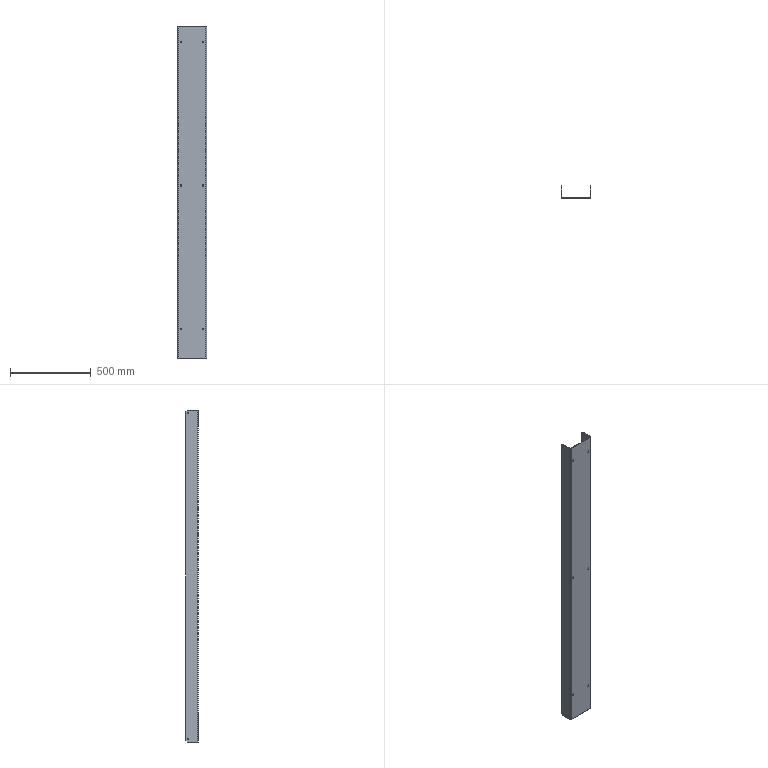Part | STEP file | HXGR200008-05-10 | 1 solid | 46 faces | box 180 x 80 x 2050 mm | volume 1362117 mm3 | cylinder 24 | plane 22 | commonest cylinder face diameters 8 x20 6 x2 10 x2
STEP:
#1=CARTESIAN_POINT('',(88.,25.,-1009.));
#2=VERTEX_POINT('',#1);
#3=CARTESIAN_POINT('',(88.,25.,-1001.));
#4=VERTEX_POINT('',#3);
#5=CARTESIAN_POINT('',(88.,25.,-1005.));
#6=DIRECTION('',(-1.,0.,0.));
#7=DIRECTION('',(0.,0.,1.));
#8=AXIS2_PLACEMENT_3D('',#5,#6,#7);
#9=CIRCLE('',#8,4.);
#10=EDGE_CURVE('',#2,#4,#9,.T.);
#11=ORIENTED_EDGE('',*,*,#10,.T.);
#12=CARTESIAN_POINT('',(90.,25.,-1001.));
#13=VERTEX_POINT('',#12);
#14=CARTESIAN_POINT('',(90.,25.,-1001.));
#15=DIRECTION('',(1.,0.,0.));
#16=VECTOR('',#15,1000.);
#17=LINE('',#14,#16);
#18=EDGE_CURVE('',#4,#13,#17,.T.);
#19=ORIENTED_EDGE('',*,*,#18,.T.);
#20=CARTESIAN_POINT('',(90.,25.,-1009.));
#21=VERTEX_POINT('',#20);
#22=CARTESIAN_POINT('',(90.,25.,-1005.));
#23=DIRECTION('',(1.,0.,0.));
#24=DIRECTION('',(0.,0.,-1.));
#25=AXIS2_PLACEMENT_3D('',#22,#23,#24);
#26=CIRCLE('',#25,4.);
#27=EDGE_CURVE('',#13,#21,#26,.T.);
#28=ORIENTED_EDGE('',*,*,#27,.T.);
#29=CARTESIAN_POINT('',(90.,25.,-1009.));
#30=DIRECTION('',(1.,0.,0.));
#31=VECTOR('',#30,1000.);
#32=LINE('',#29,#31);
#33=EDGE_CURVE('',#2,#21,#32,.T.);
#34=ORIENTED_EDGE('',*,*,#33,.F.);
#35=EDGE_LOOP('',(#11,#19,#28,#34));
#36=FACE_OUTER_BOUND('',#35,.T.);
#37=CARTESIAN_POINT('',(90.,25.,-1005.));
#38=DIRECTION('',(1.,0.,0.));
#39=DIRECTION('',(0.,0.,-1.));
#40=AXIS2_PLACEMENT_3D('',#37,#38,#39);
#41=CYLINDRICAL_SURFACE('',#40,4.);
#42=ADVANCED_FACE('',(#36),#41,.F.);
#43=CARTESIAN_POINT('',(-90.,25.,-1001.));
#44=VERTEX_POINT('',#43);
#45=CARTESIAN_POINT('',(-90.,25.,-1009.));
#46=VERTEX_POINT('',#45);
#47=CARTESIAN_POINT('',(-90.,25.,-1005.));
#48=DIRECTION('',(1.,0.,0.));
#49=DIRECTION('',(0.,0.,-1.));
#50=AXIS2_PLACEMENT_3D('',#47,#48,#49);
#51=CIRCLE('',#50,4.);
#52=EDGE_CURVE('',#44,#46,#51,.T.);
#53=ORIENTED_EDGE('',*,*,#52,.F.);
#54=CARTESIAN_POINT('',(-88.,25.,-1001.));
#55=VERTEX_POINT('',#54);
#56=CARTESIAN_POINT('',(90.,25.,-1001.));
#57=DIRECTION('',(1.,0.,0.));
#58=VECTOR('',#57,1000.);
#59=LINE('',#56,#58);
#60=EDGE_CURVE('',#44,#55,#59,.T.);
#61=ORIENTED_EDGE('',*,*,#60,.T.);
#62=CARTESIAN_POINT('',(-88.,25.,-1009.));
#63=VERTEX_POINT('',#62);
#64=CARTESIAN_POINT('',(-88.,25.,-1005.));
#65=DIRECTION('',(1.,0.,0.));
#66=DIRECTION('',(0.,0.,-1.));
#67=AXIS2_PLACEMENT_3D('',#64,#65,#66);
#68=CIRCLE('',#67,4.);
#69=EDGE_CURVE('',#55,#63,#68,.T.);
#70=ORIENTED_EDGE('',*,*,#69,.T.);
#71=CARTESIAN_POINT('',(90.,25.,-1009.));
#72=DIRECTION('',(1.,0.,0.));
#73=VECTOR('',#72,1000.);
#74=LINE('',#71,#73);
#75=EDGE_CURVE('',#46,#63,#74,.T.);
#76=ORIENTED_EDGE('',*,*,#75,.F.);
#77=EDGE_LOOP('',(#53,#61,#70,#76));
#78=FACE_OUTER_BOUND('',#77,.T.);
#79=CARTESIAN_POINT('',(90.,25.,-1005.));
#80=DIRECTION('',(1.,0.,0.));
#81=DIRECTION('',(0.,0.,-1.));
#82=AXIS2_PLACEMENT_3D('',#79,#80,#81);
#83=CYLINDRICAL_SURFACE('',#82,4.);
#84=ADVANCED_FACE('',(#78),#83,.F.);
#85=CARTESIAN_POINT('',(88.,25.,1001.));
#86=VERTEX_POINT('',#85);
#87=CARTESIAN_POINT('',(88.,25.,1009.));
#88=VERTEX_POINT('',#87);
#89=CARTESIAN_POINT('',(88.,25.,1005.));
#90=DIRECTION('',(-1.,0.,0.));
#91=DIRECTION('',(0.,0.,1.));
#92=AXIS2_PLACEMENT_3D('',#89,#90,#91);
#93=CIRCLE('',#92,4.);
#94=EDGE_CURVE('',#86,#88,#93,.T.);
#95=ORIENTED_EDGE('',*,*,#94,.T.);
#96=CARTESIAN_POINT('',(90.,25.,1009.));
#97=VERTEX_POINT('',#96);
#98=CARTESIAN_POINT('',(90.,25.,1009.));
#99=DIRECTION('',(1.,0.,0.));
#100=VECTOR('',#99,1000.);
#101=LINE('',#98,#100);
#102=EDGE_CURVE('',#88,#97,#101,.T.);
#103=ORIENTED_EDGE('',*,*,#102,.T.);
#104=CARTESIAN_POINT('',(90.,25.,1001.));
#105=VERTEX_POINT('',#104);
#106=CARTESIAN_POINT('',(90.,25.,1005.));
#107=DIRECTION('',(1.,0.,0.));
#108=DIRECTION('',(0.,0.,-1.));
#109=AXIS2_PLACEMENT_3D('',#106,#107,#108);
#110=CIRCLE('',#109,4.);
#111=EDGE_CURVE('',#97,#105,#110,.T.);
#112=ORIENTED_EDGE('',*,*,#111,.T.);
#113=CARTESIAN_POINT('',(90.,25.,1001.));
#114=DIRECTION('',(1.,0.,0.));
#115=VECTOR('',#114,1000.);
#116=LINE('',#113,#115);
#117=EDGE_CURVE('',#86,#105,#116,.T.);
#118=ORIENTED_EDGE('',*,*,#117,.F.);
#119=EDGE_LOOP('',(#95,#103,#112,#118));
#120=FACE_OUTER_BOUND('',#119,.T.);
#121=CARTESIAN_POINT('',(90.,25.,1005.));
#122=DIRECTION('',(1.,0.,0.));
#123=DIRECTION('',(0.,0.,-1.));
#124=AXIS2_PLACEMENT_3D('',#121,#122,#123);
#125=CYLINDRICAL_SURFACE('',#124,4.);
#126=ADVANCED_FACE('',(#120),#125,.F.);
#127=CARTESIAN_POINT('',(-90.,25.,1009.));
#128=VERTEX_POINT('',#127);
#129=CARTESIAN_POINT('',(-90.,25.,1001.));
#130=VERTEX_POINT('',#129);
#131=CARTESIAN_POINT('',(-90.,25.,1005.));
#132=DIRECTION('',(1.,0.,0.));
#133=DIRECTION('',(0.,0.,-1.));
#134=AXIS2_PLACEMENT_3D('',#131,#132,#133);
#135=CIRCLE('',#134,4.);
#136=EDGE_CURVE('',#128,#130,#135,.T.);
#137=ORIENTED_EDGE('',*,*,#136,.F.);
#138=CARTESIAN_POINT('',(-88.,25.,1009.));
#139=VERTEX_POINT('',#138);
#140=CARTESIAN_POINT('',(90.,25.,1009.));
#141=DIRECTION('',(1.,0.,0.));
#142=VECTOR('',#141,1000.);
#143=LINE('',#140,#142);
#144=EDGE_CURVE('',#128,#139,#143,.T.);
#145=ORIENTED_EDGE('',*,*,#144,.T.);
#146=CARTESIAN_POINT('',(-88.,25.,1001.));
#147=VERTEX_POINT('',#146);
#148=CARTESIAN_POINT('',(-88.,25.,1005.));
#149=DIRECTION('',(1.,0.,0.));
#150=DIRECTION('',(0.,0.,-1.));
#151=AXIS2_PLACEMENT_3D('',#148,#149,#150);
#152=CIRCLE('',#151,4.);
#153=EDGE_CURVE('',#139,#147,#152,.T.);
#154=ORIENTED_EDGE('',*,*,#153,.T.);
#155=CARTESIAN_POINT('',(90.,25.,1001.));
#156=DIRECTION('',(1.,0.,0.));
#157=VECTOR('',#156,1000.);
#158=LINE('',#155,#157);
#159=EDGE_CURVE('',#130,#147,#158,.T.);
#160=ORIENTED_EDGE('',*,*,#159,.F.);
#161=EDGE_LOOP('',(#137,#145,#154,#160));
#162=FACE_OUTER_BOUND('',#161,.T.);
#163=CARTESIAN_POINT('',(90.,25.,1005.));
#164=DIRECTION('',(1.,0.,0.));
#165=DIRECTION('',(0.,0.,-1.));
#166=AXIS2_PLACEMENT_3D('',#163,#164,#165);
#167=CYLINDRICAL_SURFACE('',#166,4.);
#168=ADVANCED_FACE('',(#162),#167,.F.);
#169=CARTESIAN_POINT('',(-67.5,-40.,-849.));
#170=VERTEX_POINT('',#169);
#171=CARTESIAN_POINT('',(-67.5,-40.,-841.));
#172=VERTEX_POINT('',#171);
#173=CARTESIAN_POINT('',(-67.5,-40.,-845.));
#174=DIRECTION('',(0.,1.,0.));
#175=DIRECTION('',(0.,0.,1.));
#176=AXIS2_PLACEMENT_3D('',#173,#174,#175);
#177=CIRCLE('',#176,4.);
#178=EDGE_CURVE('',#170,#172,#177,.T.);
#179=ORIENTED_EDGE('',*,*,#178,.F.);
#180=CARTESIAN_POINT('',(-67.5,-38.,-849.));
#181=VERTEX_POINT('',#180);
#182=CARTESIAN_POINT('',(-67.5,-38.,-849.));
#183=DIRECTION('',(0.,1.,0.));
#184=VECTOR('',#183,1000.);
#185=LINE('',#182,#184);
#186=EDGE_CURVE('',#170,#181,#185,.T.);
#187=ORIENTED_EDGE('',*,*,#186,.T.);
#188=CARTESIAN_POINT('',(-67.5,-38.,-841.));
#189=VERTEX_POINT('',#188);
#190=CARTESIAN_POINT('',(-67.5,-38.,-845.));
#191=DIRECTION('',(0.,1.,0.));
#192=DIRECTION('',(0.,0.,1.));
#193=AXIS2_PLACEMENT_3D('',#190,#191,#192);
#194=CIRCLE('',#193,4.);
#195=EDGE_CURVE('',#181,#189,#194,.T.);
#196=ORIENTED_EDGE('',*,*,#195,.T.);
#197=CARTESIAN_POINT('',(-67.5,-38.,-841.));
#198=DIRECTION('',(0.,1.,0.));
#199=VECTOR('',#198,1000.);
#200=LINE('',#197,#199);
#201=EDGE_CURVE('',#172,#189,#200,.T.);
#202=ORIENTED_EDGE('',*,*,#201,.F.);
#203=EDGE_LOOP('',(#179,#187,#196,#202));
#204=FACE_OUTER_BOUND('',#203,.T.);
#205=CARTESIAN_POINT('',(-67.5,-38.,-845.));
#206=DIRECTION('',(0.,1.,0.));
#207=DIRECTION('',(0.,0.,1.));
#208=AXIS2_PLACEMENT_3D('',#205,#206,#207);
#209=CYLINDRICAL_SURFACE('',#208,4.);
#210=ADVANCED_FACE('',(#204),#209,.F.);
#211=CARTESIAN_POINT('',(67.5,-40.,-849.));
#212=VERTEX_POINT('',#211);
#213=CARTESIAN_POINT('',(67.5,-40.,-841.));
#214=VERTEX_POINT('',#213);
#215=CARTESIAN_POINT('',(67.5,-40.,-845.));
#216=DIRECTION('',(0.,1.,0.));
#217=DIRECTION('',(0.,0.,1.));
#218=AXIS2_PLACEMENT_3D('',#215,#216,#217);
#219=CIRCLE('',#218,4.);
#220=EDGE_CURVE('',#212,#214,#219,.T.);
#221=ORIENTED_EDGE('',*,*,#220,.F.);
#222=CARTESIAN_POINT('',(67.5,-38.,-849.));
#223=VERTEX_POINT('',#222);
#224=CARTESIAN_POINT('',(67.5,-38.,-849.));
#225=DIRECTION('',(0.,1.,0.));
#226=VECTOR('',#225,1000.);
#227=LINE('',#224,#226);
#228=EDGE_CURVE('',#212,#223,#227,.T.);
#229=ORIENTED_EDGE('',*,*,#228,.T.);
#230=CARTESIAN_POINT('',(67.5,-38.,-841.));
#231=VERTEX_POINT('',#230);
#232=CARTESIAN_POINT('',(67.5,-38.,-845.));
#233=DIRECTION('',(0.,1.,0.));
#234=DIRECTION('',(0.,0.,1.));
#235=AXIS2_PLACEMENT_3D('',#232,#233,#234);
#236=CIRCLE('',#235,4.);
#237=EDGE_CURVE('',#223,#231,#236,.T.);
#238=ORIENTED_EDGE('',*,*,#237,.T.);
#239=CARTESIAN_POINT('',(67.5,-38.,-841.));
#240=DIRECTION('',(0.,1.,0.));
#241=VECTOR('',#240,1000.);
#242=LINE('',#239,#241);
#243=EDGE_CURVE('',#214,#231,#242,.T.);
#244=ORIENTED_EDGE('',*,*,#243,.F.);
#245=EDGE_LOOP('',(#221,#229,#238,#244));
#246=FACE_OUTER_BOUND('',#245,.T.);
#247=CARTESIAN_POINT('',(67.5,-38.,-845.));
#248=DIRECTION('',(0.,1.,0.));
#249=DIRECTION('',(0.,0.,1.));
#250=AXIS2_PLACEMENT_3D('',#247,#248,#249);
#251=CYLINDRICAL_SURFACE('',#250,4.);
#252=ADVANCED_FACE('',(#246),#251,.F.);
#253=CARTESIAN_POINT('',(-67.5,-40.,36.));
#254=VERTEX_POINT('',#253);
#255=CARTESIAN_POINT('',(-67.5,-40.,44.));
#256=VERTEX_POINT('',#255);
#257=CARTESIAN_POINT('',(-67.5,-40.,40.));
#258=DIRECTION('',(0.,1.,0.));
#259=DIRECTION('',(0.,0.,1.));
#260=AXIS2_PLACEMENT_3D('',#257,#258,#259);
#261=CIRCLE('',#260,4.);
#262=EDGE_CURVE('',#254,#256,#261,.T.);
#263=ORIENTED_EDGE('',*,*,#262,.F.);
#264=CARTESIAN_POINT('',(-67.5,-38.,36.));
#265=VERTEX_POINT('',#264);
#266=CARTESIAN_POINT('',(-67.5,-38.,36.));
#267=DIRECTION('',(0.,1.,0.));
#268=VECTOR('',#267,1000.);
#269=LINE('',#266,#268);
#270=EDGE_CURVE('',#254,#265,#269,.T.);
#271=ORIENTED_EDGE('',*,*,#270,.T.);
#272=CARTESIAN_POINT('',(-67.5,-38.,44.));
#273=VERTEX_POINT('',#272);
#274=CARTESIAN_POINT('',(-67.5,-38.,40.));
#275=DIRECTION('',(0.,1.,0.));
#276=DIRECTION('',(0.,0.,1.));
#277=AXIS2_PLACEMENT_3D('',#274,#275,#276);
#278=CIRCLE('',#277,4.);
#279=EDGE_CURVE('',#265,#273,#278,.T.);
#280=ORIENTED_EDGE('',*,*,#279,.T.);
#281=CARTESIAN_POINT('',(-67.5,-38.,44.));
#282=DIRECTION('',(0.,1.,0.));
#283=VECTOR('',#282,1000.);
#284=LINE('',#281,#283);
#285=EDGE_CURVE('',#256,#273,#284,.T.);
#286=ORIENTED_EDGE('',*,*,#285,.F.);
#287=EDGE_LOOP('',(#263,#271,#280,#286));
#288=FACE_OUTER_BOUND('',#287,.T.);
#289=CARTESIAN_POINT('',(-67.5,-38.,40.));
#290=DIRECTION('',(0.,1.,0.));
#291=DIRECTION('',(0.,0.,1.));
#292=AXIS2_PLACEMENT_3D('',#289,#290,#291);
#293=CYLINDRICAL_SURFACE('',#292,4.);
#294=ADVANCED_FACE('',(#288),#293,.F.);
#295=CARTESIAN_POINT('',(67.5,-40.,36.));
#296=VERTEX_POINT('',#295);
#297=CARTESIAN_POINT('',(67.5,-40.,44.));
#298=VERTEX_POINT('',#297);
#299=CARTESIAN_POINT('',(67.5,-40.,40.));
#300=DIRECTION('',(0.,1.,0.));
#301=DIRECTION('',(0.,0.,1.));
#302=AXIS2_PLACEMENT_3D('',#299,#300,#301);
#303=CIRCLE('',#302,4.);
#304=EDGE_CURVE('',#296,#298,#303,.T.);
#305=ORIENTED_EDGE('',*,*,#304,.F.);
#306=CARTESIAN_POINT('',(67.5,-38.,36.));
#307=VERTEX_POINT('',#306);
#308=CARTESIAN_POINT('',(67.5,-38.,36.));
#309=DIRECTION('',(0.,1.,0.));
#310=VECTOR('',#309,1000.);
#311=LINE('',#308,#310);
#312=EDGE_CURVE('',#296,#307,#311,.T.);
#313=ORIENTED_EDGE('',*,*,#312,.T.);
#314=CARTESIAN_POINT('',(67.5,-38.,44.));
#315=VERTEX_POINT('',#314);
#316=CARTESIAN_POINT('',(67.5,-38.,40.));
#317=DIRECTION('',(0.,1.,0.));
#318=DIRECTION('',(0.,0.,1.));
#319=AXIS2_PLACEMENT_3D('',#316,#317,#318);
#320=CIRCLE('',#319,4.);
#321=EDGE_CURVE('',#307,#315,#320,.T.);
#322=ORIENTED_EDGE('',*,*,#321,.T.);
#323=CARTESIAN_POINT('',(67.5,-38.,44.));
#324=DIRECTION('',(0.,1.,0.));
#325=VECTOR('',#324,1000.);
#326=LINE('',#323,#325);
#327=EDGE_CURVE('',#298,#315,#326,.T.);
#328=ORIENTED_EDGE('',*,*,#327,.F.);
#329=EDGE_LOOP('',(#305,#313,#322,#328));
#330=FACE_OUTER_BOUND('',#329,.T.);
#331=CARTESIAN_POINT('',(67.5,-38.,40.));
#332=DIRECTION('',(0.,1.,0.));
#333=DIRECTION('',(0.,0.,1.));
#334=AXIS2_PLACEMENT_3D('',#331,#332,#333);
#335=CYLINDRICAL_SURFACE('',#334,4.);
#336=ADVANCED_FACE('',(#330),#335,.F.);
#337=CARTESIAN_POINT('',(67.5,-40.,921.));
#338=VERTEX_POINT('',#337);
#339=CARTESIAN_POINT('',(67.5,-40.,929.));
#340=VERTEX_POINT('',#339);
#341=CARTESIAN_POINT('',(67.5,-40.,925.));
#342=DIRECTION('',(0.,1.,0.));
#343=DIRECTION('',(0.,0.,1.));
#344=AXIS2_PLACEMENT_3D('',#341,#342,#343);
#345=CIRCLE('',#344,4.);
#346=EDGE_CURVE('',#338,#340,#345,.T.);
#347=ORIENTED_EDGE('',*,*,#346,.F.);
#348=CARTESIAN_POINT('',(67.5,-38.,921.));
#349=VERTEX_POINT('',#348);
#350=CARTESIAN_POINT('',(67.5,-38.,921.));
#351=DIRECTION('',(0.,1.,0.));
#352=VECTOR('',#351,1000.);
#353=LINE('',#350,#352);
#354=EDGE_CURVE('',#338,#349,#353,.T.);
#355=ORIENTED_EDGE('',*,*,#354,.T.);
#356=CARTESIAN_POINT('',(67.5,-38.,929.));
#357=VERTEX_POINT('',#356);
#358=CARTESIAN_POINT('',(67.5,-38.,925.));
#359=DIRECTION('',(0.,1.,0.));
#360=DIRECTION('',(0.,0.,1.));
#361=AXIS2_PLACEMENT_3D('',#358,#359,#360);
#362=CIRCLE('',#361,4.);
#363=EDGE_CURVE('',#349,#357,#362,.T.);
#364=ORIENTED_EDGE('',*,*,#363,.T.);
#365=CARTESIAN_POINT('',(67.5,-38.,929.));
#366=DIRECTION('',(0.,1.,0.));
#367=VECTOR('',#366,1000.);
#368=LINE('',#365,#367);
#369=EDGE_CURVE('',#340,#357,#368,.T.);
#370=ORIENTED_EDGE('',*,*,#369,.F.);
#371=EDGE_LOOP('',(#347,#355,#364,#370));
#372=FACE_OUTER_BOUND('',#371,.T.);
#373=CARTESIAN_POINT('',(67.5,-38.,925.));
#374=DIRECTION('',(0.,1.,0.));
#375=DIRECTION('',(0.,0.,1.));
#376=AXIS2_PLACEMENT_3D('',#373,#374,#375);
#377=CYLINDRICAL_SURFACE('',#376,4.);
#378=ADVANCED_FACE('',(#372),#377,.F.);
#379=CARTESIAN_POINT('',(-67.5,-40.,921.));
#380=VERTEX_POINT('',#379);
#381=CARTESIAN_POINT('',(-67.5,-40.,929.));
#382=VERTEX_POINT('',#381);
#383=CARTESIAN_POINT('',(-67.5,-40.,925.));
#384=DIRECTION('',(0.,1.,0.));
#385=DIRECTION('',(0.,0.,1.));
#386=AXIS2_PLACEMENT_3D('',#383,#384,#385);
#387=CIRCLE('',#386,4.);
#388=EDGE_CURVE('',#380,#382,#387,.T.);
#389=ORIENTED_EDGE('',*,*,#388,.F.);
#390=CARTESIAN_POINT('',(-67.5,-38.,921.));
#391=VERTEX_POINT('',#390);
#392=CARTESIAN_POINT('',(-67.5,-38.,921.));
#393=DIRECTION('',(0.,1.,0.));
#394=VECTOR('',#393,1000.);
#395=LINE('',#392,#394);
#396=EDGE_CURVE('',#380,#391,#395,.T.);
#397=ORIENTED_EDGE('',*,*,#396,.T.);
#398=CARTESIAN_POINT('',(-67.5,-38.,929.));
#399=VERTEX_POINT('',#398);
#400=CARTESIAN_POINT('',(-67.5,-38.,925.));
#401=DIRECTION('',(0.,1.,0.));
#402=DIRECTION('',(0.,0.,1.));
#403=AXIS2_PLACEMENT_3D('',#400,#401,#402);
#404=CIRCLE('',#403,4.);
#405=EDGE_CURVE('',#391,#399,#404,.T.);
#406=ORIENTED_EDGE('',*,*,#405,.T.);
#407=CARTESIAN_POINT('',(-67.5,-38.,929.));
#408=DIRECTION('',(0.,1.,0.));
#409=VECTOR('',#408,1000.);
#410=LINE('',#407,#409);
#411=EDGE_CURVE('',#382,#399,#410,.T.);
#412=ORIENTED_EDGE('',*,*,#411,.F.);
#413=EDGE_LOOP('',(#389,#397,#406,#412));
#414=FACE_OUTER_BOUND('',#413,.T.);
#415=CARTESIAN_POINT('',(-67.5,-38.,925.));
#416=DIRECTION('',(0.,1.,0.));
#417=DIRECTION('',(0.,0.,1.));
#418=AXIS2_PLACEMENT_3D('',#415,#416,#417);
#419=CYLINDRICAL_SURFACE('',#418,4.);
#420=ADVANCED_FACE('',(#414),#419,.F.);
#421=CARTESIAN_POINT('',(-90.,-35.,1025.));
#422=VERTEX_POINT('',#421);
#423=CARTESIAN_POINT('',(-88.,-35.,1025.));
#424=VERTEX_POINT('',#423);
#425=CARTESIAN_POINT('',(-90.,-35.,1025.));
#426=DIRECTION('',(1.,0.,0.));
#427=VECTOR('',#426,1000.);
#428=LINE('',#425,#427);
#429=EDGE_CURVE('',#422,#424,#428,.T.);
#430=ORIENTED_EDGE('',*,*,#429,.F.);
#431=CARTESIAN_POINT('',(-85.,-40.,1025.));
#432=VERTEX_POINT('',#431);
#433=CARTESIAN_POINT('',(-85.,-35.,1025.));
#434=DIRECTION('',(0.,0.,1.));
#435=DIRECTION('',(-1.,0.,0.));
#436=AXIS2_PLACEMENT_3D('',#433,#434,#435);
#437=CIRCLE('',#436,5.);
#438=EDGE_CURVE('',#422,#432,#437,.T.);
#439=ORIENTED_EDGE('',*,*,#438,.T.);
#440=CARTESIAN_POINT('',(-85.,-38.,1025.));
#441=VERTEX_POINT('',#440);
#442=CARTESIAN_POINT('',(-85.,-38.,1025.));
#443=DIRECTION('',(0.,-1.,0.));
#444=VECTOR('',#443,1000.);
#445=LINE('',#442,#444);
#446=EDGE_CURVE('',#441,#432,#445,.T.);
#447=ORIENTED_EDGE('',*,*,#446,.F.);
#448=CARTESIAN_POINT('',(-85.,-35.,1025.));
#449=DIRECTION('',(0.,0.,1.));
#450=DIRECTION('',(1.,0.,0.));
#451=AXIS2_PLACEMENT_3D('',#448,#449,#450);
#452=CIRCLE('',#451,3.);
#453=EDGE_CURVE('',#424,#441,#452,.T.);
#454=ORIENTED_EDGE('',*,*,#453,.F.);
#455=EDGE_LOOP('',(#430,#439,#447,#454));
#456=FACE_OUTER_BOUND('',#455,.T.);
#457=CARTESIAN_POINT('',(-90.,-35.,1025.));
#458=DIRECTION('',(0.,0.,1.));
#459=DIRECTION('',(1.,0.,0.));
#460=AXIS2_PLACEMENT_3D('',#457,#458,#459);
#461=PLANE('',#460);
#462=ADVANCED_FACE('',(#456),#461,.T.);
#463=CARTESIAN_POINT('',(-88.,30.,1025.));
#464=VERTEX_POINT('',#463);
#465=CARTESIAN_POINT('',(-88.,-40.,1025.));
#466=DIRECTION('',(0.,-1.,0.));
#467=VECTOR('',#466,1000.);
#468=LINE('',#465,#467);
#469=EDGE_CURVE('',#464,#424,#468,.T.);
#470=ORIENTED_EDGE('',*,*,#469,.F.);
#471=CARTESIAN_POINT('',(-90.,30.,1025.));
#472=VERTEX_POINT('',#471);
#473=CARTESIAN_POINT('',(-85.,30.,1025.));
#474=DIRECTION('',(-1.,0.,0.));
#475=VECTOR('',#474,1000.);
#476=LINE('',#473,#475);
#477=EDGE_CURVE('',#464,#472,#476,.T.);
#478=ORIENTED_EDGE('',*,*,#477,.T.);
#479=CARTESIAN_POINT('',(-90.,-40.,1025.));
#480=DIRECTION('',(0.,-1.,0.));
#481=VECTOR('',#480,1000.);
#482=LINE('',#479,#481);
#483=EDGE_CURVE('',#472,#422,#482,.T.);
#484=ORIENTED_EDGE('',*,*,#483,.T.);
#485=ORIENTED_EDGE('',*,*,#429,.T.);
#486=EDGE_LOOP('',(#470,#478,#484,#485));
#487=FACE_OUTER_BOUND('',#486,.T.);
#488=CARTESIAN_POINT('',(-85.,-38.,1025.));
#489=DIRECTION('',(0.,0.,1.));
#490=DIRECTION('',(1.,0.,0.));
#491=AXIS2_PLACEMENT_3D('',#488,#489,#490);
#492=PLANE('',#491);
#493=ADVANCED_FACE('',(#487),#492,.T.);
#494=CARTESIAN_POINT('',(-85.,-40.,-1025.));
#495=VERTEX_POINT('',#494);
#496=CARTESIAN_POINT('',(-85.,-38.,-1025.));
#497=VERTEX_POINT('',#496);
#498=CARTESIAN_POINT('',(-85.,-40.,-1025.));
#499=DIRECTION('',(0.,1.,0.));
#500=VECTOR('',#499,1000.);
#501=LINE('',#498,#500);
#502=EDGE_CURVE('',#495,#497,#501,.T.);
#503=ORIENTED_EDGE('',*,*,#502,.F.);
#504=CARTESIAN_POINT('',(-90.,-35.,-1025.));
#505=VERTEX_POINT('',#504);
#506=CARTESIAN_POINT('',(-85.,-35.,-1025.));
#507=DIRECTION('',(0.,0.,1.));
#508=DIRECTION('',(-1.,0.,0.));
#509=AXIS2_PLACEMENT_3D('',#506,#507,#508);
#510=CIRCLE('',#509,5.);
#511=EDGE_CURVE('',#505,#495,#510,.T.);
#512=ORIENTED_EDGE('',*,*,#511,.F.);
#513=CARTESIAN_POINT('',(-88.,-35.,-1025.));
#514=VERTEX_POINT('',#513);
#515=CARTESIAN_POINT('',(-88.,-35.,-1025.));
#516=DIRECTION('',(-1.,0.,0.));
#517=VECTOR('',#516,1000.);
#518=LINE('',#515,#517);
#519=EDGE_CURVE('',#514,#505,#518,.T.);
#520=ORIENTED_EDGE('',*,*,#519,.F.);
#521=CARTESIAN_POINT('',(-85.,-35.,-1025.));
#522=DIRECTION('',(0.,0.,1.));
#523=DIRECTION('',(1.,0.,0.));
#524=AXIS2_PLACEMENT_3D('',#521,#522,#523);
#525=CIRCLE('',#524,3.);
#526=EDGE_CURVE('',#514,#497,#525,.T.);
#527=ORIENTED_EDGE('',*,*,#526,.T.);
#528=EDGE_LOOP('',(#503,#512,#520,#527));
#529=FACE_OUTER_BOUND('',#528,.T.);
#530=CARTESIAN_POINT('',(-85.,-40.,-1025.));
#531=DIRECTION('',(0.,0.,-1.));
#532=DIRECTION('',(-1.,0.,0.));
#533=AXIS2_PLACEMENT_3D('',#530,#531,#532);
#534=PLANE('',#533);
#535=ADVANCED_FACE('',(#529),#534,.T.);
#536=CARTESIAN_POINT('',(85.,-40.,-1025.));
#537=VERTEX_POINT('',#536);
#538=CARTESIAN_POINT('',(90.,-40.,-1025.));
#539=DIRECTION('',(1.,0.,0.));
#540=VECTOR('',#539,1000.);
#541=LINE('',#538,#540);
#542=EDGE_CURVE('',#495,#537,#541,.T.);
#543=ORIENTED_EDGE('',*,*,#542,.F.);
#544=ORIENTED_EDGE('',*,*,#502,.T.);
#545=CARTESIAN_POINT('',(85.,-38.,-1025.));
#546=VERTEX_POINT('',#545);
#547=CARTESIAN_POINT('',(90.,-38.,-1025.));
#548=DIRECTION('',(1.,0.,0.));
#549=VECTOR('',#548,1000.);
#550=LINE('',#547,#549);
#551=EDGE_CURVE('',#497,#546,#550,.T.);
#552=ORIENTED_EDGE('',*,*,#551,.T.);
#553=CARTESIAN_POINT('',(85.,-38.,-1025.));
#554=DIRECTION('',(0.,-1.,0.));
#555=VECTOR('',#554,1000.);
#556=LINE('',#553,#555);
#557=EDGE_CURVE('',#546,#537,#556,.T.);
#558=ORIENTED_EDGE('',*,*,#557,.T.);
#559=EDGE_LOOP('',(#543,#544,#552,#558));
#560=FACE_OUTER_BOUND('',#559,.T.);
#561=CARTESIAN_POINT('',(-88.,-35.,-1025.));
#562=DIRECTION('',(0.,0.,-1.));
#563=DIRECTION('',(-1.,0.,0.));
#564=AXIS2_PLACEMENT_3D('',#561,#562,#563);
#565=PLANE('',#564);
#566=ADVANCED_FACE('',(#560),#565,.T.);
#567=CARTESIAN_POINT('',(85.,-40.,1025.));
#568=VERTEX_POINT('',#567);
#569=CARTESIAN_POINT('',(85.,-38.,1025.));
#570=VERTEX_POINT('',#569);
#571=CARTESIAN_POINT('',(85.,-40.,1025.));
#572=DIRECTION('',(0.,1.,0.));
#573=VECTOR('',#572,1000.);
#574=LINE('',#571,#573);
#575=EDGE_CURVE('',#568,#570,#574,.T.);
#576=ORIENTED_EDGE('',*,*,#575,.F.);
#577=CARTESIAN_POINT('',(90.,-35.,1025.));
#578=VERTEX_POINT('',#577);
#579=CARTESIAN_POINT('',(85.,-35.,1025.));
#580=DIRECTION('',(0.,0.,1.));
#581=DIRECTION('',(-1.,0.,0.));
#582=AXIS2_PLACEMENT_3D('',#579,#580,#581);
#583=CIRCLE('',#582,5.);
#584=EDGE_CURVE('',#568,#578,#583,.T.);
#585=ORIENTED_EDGE('',*,*,#584,.T.);
#586=CARTESIAN_POINT('',(88.,-35.,1025.));
#587=VERTEX_POINT('',#586);
#588=CARTESIAN_POINT('',(88.,-35.,1025.));
#589=DIRECTION('',(1.,0.,0.));
#590=VECTOR('',#589,1000.);
#591=LINE('',#588,#590);
#592=EDGE_CURVE('',#587,#578,#591,.T.);
#593=ORIENTED_EDGE('',*,*,#592,.F.);
#594=CARTESIAN_POINT('',(85.,-35.,1025.));
#595=DIRECTION('',(0.,0.,1.));
#596=DIRECTION('',(1.,0.,0.));
#597=AXIS2_PLACEMENT_3D('',#594,#595,#596);
#598=CIRCLE('',#597,3.);
#599=EDGE_CURVE('',#570,#587,#598,.T.);
#600=ORIENTED_EDGE('',*,*,#599,.F.);
#601=EDGE_LOOP('',(#576,#585,#593,#600));
#602=FACE_OUTER_BOUND('',#601,.T.);
#603=CARTESIAN_POINT('',(85.,-40.,1025.));
#604=DIRECTION('',(0.,0.,1.));
#605=DIRECTION('',(1.,0.,0.));
#606=AXIS2_PLACEMENT_3D('',#603,#604,#605);
#607=PLANE('',#606);
#608=ADVANCED_FACE('',(#602),#607,.T.);
#609=CARTESIAN_POINT('',(90.,-40.,1025.));
#610=DIRECTION('',(1.,0.,0.));
#611=VECTOR('',#610,1000.);
#612=LINE('',#609,#611);
#613=EDGE_CURVE('',#432,#568,#612,.T.);
#614=ORIENTED_EDGE('',*,*,#613,.T.);
#615=ORIENTED_EDGE('',*,*,#575,.T.);
#616=CARTESIAN_POINT('',(90.,-38.,1025.));
#617=DIRECTION('',(1.,0.,0.));
#618=VECTOR('',#617,1000.);
#619=LINE('',#616,#618);
#620=EDGE_CURVE('',#441,#570,#619,.T.);
#621=ORIENTED_EDGE('',*,*,#620,.F.);
#622=ORIENTED_EDGE('',*,*,#446,.T.);
#623=EDGE_LOOP('',(#614,#615,#621,#622));
#624=FACE_OUTER_BOUND('',#623,.T.);
#625=CARTESIAN_POINT('',(88.,-35.,1025.));
#626=DIRECTION('',(0.,0.,1.));
#627=DIRECTION('',(1.,0.,0.));
#628=AXIS2_PLACEMENT_3D('',#625,#626,#627);
#629=PLANE('',#628);
#630=ADVANCED_FACE('',(#624),#629,.T.);
#631=CARTESIAN_POINT('',(90.,-35.,-1025.));
#632=VERTEX_POINT('',#631);
#633=CARTESIAN_POINT('',(88.,-35.,-1025.));
#634=VERTEX_POINT('',#633);
#635=CARTESIAN_POINT('',(90.,-35.,-1025.));
#636=DIRECTION('',(-1.,0.,0.));
#637=VECTOR('',#636,1000.);
#638=LINE('',#635,#637);
#639=EDGE_CURVE('',#632,#634,#638,.T.);
#640=ORIENTED_EDGE('',*,*,#639,.F.);
#641=CARTESIAN_POINT('',(85.,-35.,-1025.));
#642=DIRECTION('',(0.,0.,1.));
#643=DIRECTION('',(-1.,0.,0.));
#644=AXIS2_PLACEMENT_3D('',#641,#642,#643);
#645=CIRCLE('',#644,5.);
#646=EDGE_CURVE('',#537,#632,#645,.T.);
#647=ORIENTED_EDGE('',*,*,#646,.F.);
#648=ORIENTED_EDGE('',*,*,#557,.F.);
#649=CARTESIAN_POINT('',(85.,-35.,-1025.));
#650=DIRECTION('',(0.,0.,1.));
#651=DIRECTION('',(1.,0.,0.));
#652=AXIS2_PLACEMENT_3D('',#649,#650,#651);
#653=CIRCLE('',#652,3.);
#654=EDGE_CURVE('',#546,#634,#653,.T.);
#655=ORIENTED_EDGE('',*,*,#654,.T.);
#656=EDGE_LOOP('',(#640,#647,#648,#655));
#657=FACE_OUTER_BOUND('',#656,.T.);
#658=CARTESIAN_POINT('',(90.,-35.,-1025.));
#659=DIRECTION('',(0.,0.,-1.));
#660=DIRECTION('',(-1.,0.,0.));
#661=AXIS2_PLACEMENT_3D('',#658,#659,#660);
#662=PLANE('',#661);
#663=ADVANCED_FACE('',(#657),#662,.T.);
#664=CARTESIAN_POINT('',(88.,30.,-1025.));
#665=VERTEX_POINT('',#664);
#666=CARTESIAN_POINT('',(88.,-40.,-1025.));
#667=DIRECTION('',(0.,1.,0.));
#668=VECTOR('',#667,1000.);
#669=LINE('',#666,#668);
#670=EDGE_CURVE('',#634,#665,#669,.T.);
#671=ORIENTED_EDGE('',*,*,#670,.T.);
#672=CARTESIAN_POINT('',(90.,30.,-1025.));
#673=VERTEX_POINT('',#672);
#674=CARTESIAN_POINT('',(85.,30.,-1025.));
#675=DIRECTION('',(1.,0.,0.));
#676=VECTOR('',#675,1000.);
#677=LINE('',#674,#676);
#678=EDGE_CURVE('',#665,#673,#677,.T.);
#679=ORIENTED_EDGE('',*,*,#678,.T.);
#680=CARTESIAN_POINT('',(90.,-40.,-1025.));
#681=DIRECTION('',(0.,1.,0.));
#682=VECTOR('',#681,1000.);
#683=LINE('',#680,#682);
#684=EDGE_CURVE('',#632,#673,#683,.T.);
#685=ORIENTED_EDGE('',*,*,#684,.F.);
#686=ORIENTED_EDGE('',*,*,#639,.T.);
#687=EDGE_LOOP('',(#671,#679,#685,#686));
#688=FACE_OUTER_BOUND('',#687,.T.);
#689=CARTESIAN_POINT('',(85.,-38.,-1025.));
#690=DIRECTION('',(0.,0.,-1.));
#691=DIRECTION('',(-1.,0.,0.));
#692=AXIS2_PLACEMENT_3D('',#689,#690,#691);
#693=PLANE('',#692);
#694=ADVANCED_FACE('',(#688),#693,.T.);
#695=CARTESIAN_POINT('',(90.,25.,-1005.));
#696=DIRECTION('',(1.,0.,0.));
#697=DIRECTION('',(0.,0.,-1.));
#698=AXIS2_PLACEMENT_3D('',#695,#696,#697);
#699=CIRCLE('',#698,4.);
#700=EDGE_CURVE('',#21,#13,#699,.T.);
#701=ORIENTED_EDGE('',*,*,#700,.F.);
#702=ORIENTED_EDGE('',*,*,#27,.F.);
#703=EDGE_LOOP('',(#701,#702));
#704=FACE_BOUND('',#703,.T.);
#705=CARTESIAN_POINT('',(90.,25.,1005.));
#706=DIRECTION('',(1.,0.,0.));
#707=DIRECTION('',(0.,0.,-1.));
#708=AXIS2_PLACEMENT_3D('',#705,#706,#707);
#709=CIRCLE('',#708,4.);
#710=EDGE_CURVE('',#105,#97,#709,.T.);
#711=ORIENTED_EDGE('',*,*,#710,.F.);
#712=ORIENTED_EDGE('',*,*,#111,.F.);
#713=EDGE_LOOP('',(#711,#712));
#714=FACE_BOUND('',#713,.T.);
#715=CARTESIAN_POINT('',(90.,40.,1015.));
#716=VERTEX_POINT('',#715);
#717=CARTESIAN_POINT('',(90.,40.,-1015.));
#718=VERTEX_POINT('',#717);
#719=CARTESIAN_POINT('',(90.,40.,1025.));
#720=DIRECTION('',(0.,0.,-1.));
#721=VECTOR('',#720,1000.);
#722=LINE('',#719,#721);
#723=EDGE_CURVE('',#716,#718,#722,.T.);
#724=ORIENTED_EDGE('',*,*,#723,.F.);
#725=CARTESIAN_POINT('',(90.,30.,1025.));
#726=VERTEX_POINT('',#725);
#727=CARTESIAN_POINT('',(90.,40.,1015.));
#728=DIRECTION('',(0.,-0.7071,0.7071));
#729=VECTOR('',#728,1000.);
#730=LINE('',#727,#729);
#731=EDGE_CURVE('',#716,#726,#730,.T.);
#732=ORIENTED_EDGE('',*,*,#731,.T.);
#733=CARTESIAN_POINT('',(90.,-40.,1025.));
#734=DIRECTION('',(0.,1.,0.));
#735=VECTOR('',#734,1000.);
#736=LINE('',#733,#735);
#737=EDGE_CURVE('',#578,#726,#736,.T.);
#738=ORIENTED_EDGE('',*,*,#737,.F.);
#739=CARTESIAN_POINT('',(90.,-35.,1025.));
#740=DIRECTION('',(0.,0.,-1.));
#741=VECTOR('',#740,1000.);
#742=LINE('',#739,#741);
#743=EDGE_CURVE('',#578,#632,#742,.T.);
#744=ORIENTED_EDGE('',*,*,#743,.T.);
#745=ORIENTED_EDGE('',*,*,#684,.T.);
#746=CARTESIAN_POINT('',(90.,30.,-1025.));
#747=DIRECTION('',(0.,0.7071,0.7071));
#748=VECTOR('',#747,1000.);
#749=LINE('',#746,#748);
#750=EDGE_CURVE('',#673,#718,#749,.T.);
#751=ORIENTED_EDGE('',*,*,#750,.T.);
#752=EDGE_LOOP('',(#724,#732,#738,#744,#745,#751));
#753=FACE_OUTER_BOUND('',#752,.T.);
#754=CARTESIAN_POINT('',(90.,-40.,1025.));
#755=DIRECTION('',(-1.,0.,0.));
#756=DIRECTION('',(0.,0.,1.));
#757=AXIS2_PLACEMENT_3D('',#754,#755,#756);
#758=PLANE('',#757);
#759=ADVANCED_FACE('',(#704,#714,#753),#758,.F.);
#760=CARTESIAN_POINT('',(88.,40.,1015.));
#761=VERTEX_POINT('',#760);
#762=CARTESIAN_POINT('',(88.,40.,-1015.));
#763=VERTEX_POINT('',#762);
#764=CARTESIAN_POINT('',(88.,40.,1025.));
#765=DIRECTION('',(0.,0.,-1.));
#766=VECTOR('',#765,1000.);
#767=LINE('',#764,#766);
#768=EDGE_CURVE('',#761,#763,#767,.T.);
#769=ORIENTED_EDGE('',*,*,#768,.F.);
#770=CARTESIAN_POINT('',(88.,40.,1015.));
#771=DIRECTION('',(1.,0.,0.));
#772=VECTOR('',#771,1000.);
#773=LINE('',#770,#772);
#774=EDGE_CURVE('',#761,#716,#773,.T.);
#775=ORIENTED_EDGE('',*,*,#774,.T.);
#776=ORIENTED_EDGE('',*,*,#723,.T.);
#777=CARTESIAN_POINT('',(88.,40.,-1015.));
#778=DIRECTION('',(-1.,0.,0.));
#779=VECTOR('',#778,1000.);
#780=LINE('',#777,#779);
#781=EDGE_CURVE('',#718,#763,#780,.T.);
#782=ORIENTED_EDGE('',*,*,#781,.T.);
#783=EDGE_LOOP('',(#769,#775,#776,#782));
#784=FACE_OUTER_BOUND('',#783,.T.);
#785=CARTESIAN_POINT('',(88.,40.,1025.));
#786=DIRECTION('',(0.,1.,0.));
#787=DIRECTION('',(0.,0.,1.));
#788=AXIS2_PLACEMENT_3D('',#785,#786,#787);
#789=PLANE('',#788);
#790=ADVANCED_FACE('',(#784),#789,.T.);
#791=ORIENTED_EDGE('',*,*,#10,.F.);
#792=CARTESIAN_POINT('',(88.,25.,-1005.));
#793=DIRECTION('',(-1.,0.,0.));
#794=DIRECTION('',(0.,0.,1.));
#795=AXIS2_PLACEMENT_3D('',#792,#793,#794);
#796=CIRCLE('',#795,4.);
#797=EDGE_CURVE('',#4,#2,#796,.T.);
#798=ORIENTED_EDGE('',*,*,#797,.F.);
#799=EDGE_LOOP('',(#791,#798));
#800=FACE_BOUND('',#799,.T.);
#801=ORIENTED_EDGE('',*,*,#94,.F.);
#802=CARTESIAN_POINT('',(88.,25.,1005.));
#803=DIRECTION('',(-1.,0.,0.));
#804=DIRECTION('',(0.,0.,1.));
#805=AXIS2_PLACEMENT_3D('',#802,#803,#804);
#806=CIRCLE('',#805,4.);
#807=EDGE_CURVE('',#88,#86,#806,.T.);
#808=ORIENTED_EDGE('',*,*,#807,.F.);
#809=EDGE_LOOP('',(#801,#808));
#810=FACE_BOUND('',#809,.T.);
#811=CARTESIAN_POINT('',(88.,30.,1025.));
#812=VERTEX_POINT('',#811);
#813=CARTESIAN_POINT('',(88.,-40.,1025.));
#814=DIRECTION('',(0.,1.,0.));
#815=VECTOR('',#814,1000.);
#816=LINE('',#813,#815);
#817=EDGE_CURVE('',#587,#812,#816,.T.);
#818=ORIENTED_EDGE('',*,*,#817,.T.);
#819=CARTESIAN_POINT('',(88.,-5.,1060.));
#820=DIRECTION('',(0.,0.7071,-0.7071));
#821=VECTOR('',#820,1000.);
#822=LINE('',#819,#821);
#823=EDGE_CURVE('',#812,#761,#822,.T.);
#824=ORIENTED_EDGE('',*,*,#823,.T.);
#825=ORIENTED_EDGE('',*,*,#768,.T.);
#826=CARTESIAN_POINT('',(88.,1020.,-35.));
#827=DIRECTION('',(0.,-0.7071,-0.7071));
#828=VECTOR('',#827,1000.);
#829=LINE('',#826,#828);
#830=EDGE_CURVE('',#763,#665,#829,.T.);
#831=ORIENTED_EDGE('',*,*,#830,.T.);
#832=ORIENTED_EDGE('',*,*,#670,.F.);
#833=CARTESIAN_POINT('',(88.,-35.,1025.));
#834=DIRECTION('',(0.,0.,-1.));
#835=VECTOR('',#834,1000.);
#836=LINE('',#833,#835);
#837=EDGE_CURVE('',#587,#634,#836,.T.);
#838=ORIENTED_EDGE('',*,*,#837,.F.);
#839=EDGE_LOOP('',(#818,#824,#825,#831,#832,#838));
#840=FACE_OUTER_BOUND('',#839,.T.);
#841=CARTESIAN_POINT('',(88.,-40.,1025.));
#842=DIRECTION('',(-1.,0.,0.));
#843=DIRECTION('',(0.,0.,1.));
#844=AXIS2_PLACEMENT_3D('',#841,#842,#843);
#845=PLANE('',#844);
#846=ADVANCED_FACE('',(#800,#810,#840),#845,.T.);
#847=ORIENTED_EDGE('',*,*,#654,.F.);
#848=CARTESIAN_POINT('',(85.,-38.,1025.));
#849=DIRECTION('',(0.,0.,-1.));
#850=VECTOR('',#849,1000.);
#851=LINE('',#848,#850);
#852=EDGE_CURVE('',#570,#546,#851,.T.);
#853=ORIENTED_EDGE('',*,*,#852,.F.);
#854=ORIENTED_EDGE('',*,*,#599,.T.);
#855=ORIENTED_EDGE('',*,*,#837,.T.);
#856=EDGE_LOOP('',(#847,#853,#854,#855));
#857=FACE_OUTER_BOUND('',#856,.T.);
#858=CARTESIAN_POINT('',(85.,-35.,1025.));
#859=DIRECTION('',(0.,0.,-1.));
#860=DIRECTION('',(-1.,0.,0.));
#861=AXIS2_PLACEMENT_3D('',#858,#859,#860);
#862=CYLINDRICAL_SURFACE('',#861,3.);
#863=ADVANCED_FACE('',(#857),#862,.F.);
#864=CARTESIAN_POINT('',(-67.5,-38.,-845.));
#865=DIRECTION('',(0.,1.,0.));
#866=DIRECTION('',(0.,0.,1.));
#867=AXIS2_PLACEMENT_3D('',#864,#865,#866);
#868=CIRCLE('',#867,4.);
#869=EDGE_CURVE('',#189,#181,#868,.T.);
#870=ORIENTED_EDGE('',*,*,#869,.F.);
#871=ORIENTED_EDGE('',*,*,#195,.F.);
#872=EDGE_LOOP('',(#870,#871));
#873=FACE_BOUND('',#872,.T.);
#874=CARTESIAN_POINT('',(67.5,-38.,-845.));
#875=DIRECTION('',(0.,1.,0.));
#876=DIRECTION('',(0.,0.,1.));
#877=AXIS2_PLACEMENT_3D('',#874,#875,#876);
#878=CIRCLE('',#877,4.);
#879=EDGE_CURVE('',#231,#223,#878,.T.);
#880=ORIENTED_EDGE('',*,*,#879,.F.);
#881=ORIENTED_EDGE('',*,*,#237,.F.);
#882=EDGE_LOOP('',(#880,#881));
#883=FACE_BOUND('',#882,.T.);
#884=CARTESIAN_POINT('',(-67.5,-38.,40.));
#885=DIRECTION('',(0.,1.,0.));
#886=DIRECTION('',(0.,0.,1.));
#887=AXIS2_PLACEMENT_3D('',#884,#885,#886);
#888=CIRCLE('',#887,4.);
#889=EDGE_CURVE('',#273,#265,#888,.T.);
#890=ORIENTED_EDGE('',*,*,#889,.F.);
#891=ORIENTED_EDGE('',*,*,#279,.F.);
#892=EDGE_LOOP('',(#890,#891));
#893=FACE_BOUND('',#892,.T.);
#894=CARTESIAN_POINT('',(67.5,-38.,40.));
#895=DIRECTION('',(0.,1.,0.));
#896=DIRECTION('',(0.,0.,1.));
#897=AXIS2_PLACEMENT_3D('',#894,#895,#896);
#898=CIRCLE('',#897,4.);
#899=EDGE_CURVE('',#315,#307,#898,.T.);
#900=ORIENTED_EDGE('',*,*,#899,.F.);
#901=ORIENTED_EDGE('',*,*,#321,.F.);
#902=EDGE_LOOP('',(#900,#901));
#903=FACE_BOUND('',#902,.T.);
#904=CARTESIAN_POINT('',(67.5,-38.,925.));
#905=DIRECTION('',(0.,1.,0.));
#906=DIRECTION('',(0.,0.,1.));
#907=AXIS2_PLACEMENT_3D('',#904,#905,#906);
#908=CIRCLE('',#907,4.);
#909=EDGE_CURVE('',#357,#349,#908,.T.);
#910=ORIENTED_EDGE('',*,*,#909,.F.);
#911=ORIENTED_EDGE('',*,*,#363,.F.);
#912=EDGE_LOOP('',(#910,#911));
#913=FACE_BOUND('',#912,.T.);
#914=CARTESIAN_POINT('',(-67.5,-38.,925.));
#915=DIRECTION('',(0.,1.,0.));
#916=DIRECTION('',(0.,0.,1.));
#917=AXIS2_PLACEMENT_3D('',#914,#915,#916);
#918=CIRCLE('',#917,4.);
#919=EDGE_CURVE('',#399,#391,#918,.T.);
#920=ORIENTED_EDGE('',*,*,#919,.F.);
#921=ORIENTED_EDGE('',*,*,#405,.F.);
#922=EDGE_LOOP('',(#920,#921));
#923=FACE_BOUND('',#922,.T.);
#924=ORIENTED_EDGE('',*,*,#551,.F.);
#925=CARTESIAN_POINT('',(-85.,-38.,1025.));
#926=DIRECTION('',(0.,0.,-1.));
#927=VECTOR('',#926,1000.);
#928=LINE('',#925,#927);
#929=EDGE_CURVE('',#441,#497,#928,.T.);
#930=ORIENTED_EDGE('',*,*,#929,.F.);
#931=ORIENTED_EDGE('',*,*,#620,.T.);
#932=ORIENTED_EDGE('',*,*,#852,.T.);
#933=EDGE_LOOP('',(#924,#930,#931,#932));
#934=FACE_OUTER_BOUND('',#933,.T.);
#935=CARTESIAN_POINT('',(90.,-38.,1025.));
#936=DIRECTION('',(0.,1.,0.));
#937=DIRECTION('',(-1.,0.,0.));
#938=AXIS2_PLACEMENT_3D('',#935,#936,#937);
#939=PLANE('',#938);
#940=ADVANCED_FACE('',(#873,#883,#893,#903,#913,#923,#934),#939,.T.);
#941=ORIENTED_EDGE('',*,*,#526,.F.);
#942=CARTESIAN_POINT('',(-88.,-35.,1025.));
#943=DIRECTION('',(0.,0.,-1.));
#944=VECTOR('',#943,1000.);
#945=LINE('',#942,#944);
#946=EDGE_CURVE('',#424,#514,#945,.T.);
#947=ORIENTED_EDGE('',*,*,#946,.F.);
#948=ORIENTED_EDGE('',*,*,#453,.T.);
#949=ORIENTED_EDGE('',*,*,#929,.T.);
#950=EDGE_LOOP('',(#941,#947,#948,#949));
#951=FACE_OUTER_BOUND('',#950,.T.);
#952=CARTESIAN_POINT('',(-85.,-35.,1025.));
#953=DIRECTION('',(0.,0.,-1.));
#954=DIRECTION('',(-1.,0.,0.));
#955=AXIS2_PLACEMENT_3D('',#952,#953,#954);
#956=CYLINDRICAL_SURFACE('',#955,3.);
#957=ADVANCED_FACE('',(#951),#956,.F.);
#958=CARTESIAN_POINT('',(-88.,25.,-1005.));
#959=DIRECTION('',(1.,0.,0.));
#960=DIRECTION('',(0.,0.,-1.));
#961=AXIS2_PLACEMENT_3D('',#958,#959,#960);
#962=CIRCLE('',#961,4.);
#963=EDGE_CURVE('',#63,#55,#962,.T.);
#964=ORIENTED_EDGE('',*,*,#963,.F.);
#965=ORIENTED_EDGE('',*,*,#69,.F.);
#966=EDGE_LOOP('',(#964,#965));
#967=FACE_BOUND('',#966,.T.);
#968=CARTESIAN_POINT('',(-88.,25.,1005.));
#969=DIRECTION('',(1.,0.,0.));
#970=DIRECTION('',(0.,0.,-1.));
#971=AXIS2_PLACEMENT_3D('',#968,#969,#970);
#972=CIRCLE('',#971,4.);
#973=EDGE_CURVE('',#147,#139,#972,.T.);
#974=ORIENTED_EDGE('',*,*,#973,.F.);
#975=ORIENTED_EDGE('',*,*,#153,.F.);
#976=EDGE_LOOP('',(#974,#975));
#977=FACE_BOUND('',#976,.T.);
#978=CARTESIAN_POINT('',(-88.,40.,1015.));
#979=VERTEX_POINT('',#978);
#980=CARTESIAN_POINT('',(-88.,40.,-1015.));
#981=VERTEX_POINT('',#980);
#982=CARTESIAN_POINT('',(-88.,40.,1025.));
#983=DIRECTION('',(0.,0.,-1.));
#984=VECTOR('',#983,1000.);
#985=LINE('',#982,#984);
#986=EDGE_CURVE('',#979,#981,#985,.T.);
#987=ORIENTED_EDGE('',*,*,#986,.F.);
#988=CARTESIAN_POINT('',(-88.,-5.,1060.));
#989=DIRECTION('',(0.,-0.7071,0.7071));
#990=VECTOR('',#989,1000.);
#991=LINE('',#988,#990);
#992=EDGE_CURVE('',#979,#464,#991,.T.);
#993=ORIENTED_EDGE('',*,*,#992,.T.);
#994=ORIENTED_EDGE('',*,*,#469,.T.);
#995=ORIENTED_EDGE('',*,*,#946,.T.);
#996=CARTESIAN_POINT('',(-88.,30.,-1025.));
#997=VERTEX_POINT('',#996);
#998=CARTESIAN_POINT('',(-88.,-40.,-1025.));
#999=DIRECTION('',(0.,-1.,0.));
#1000=VECTOR('',#999,1000.);
#1001=LINE('',#998,#1000);
#1002=EDGE_CURVE('',#997,#514,#1001,.T.);
#1003=ORIENTED_EDGE('',*,*,#1002,.F.);
#1004=CARTESIAN_POINT('',(-88.,1020.,-35.));
#1005=DIRECTION('',(0.,0.7071,0.7071));
#1006=VECTOR('',#1005,1000.);
#1007=LINE('',#1004,#1006);
#1008=EDGE_CURVE('',#997,#981,#1007,.T.);
#1009=ORIENTED_EDGE('',*,*,#1008,.T.);
#1010=EDGE_LOOP('',(#987,#993,#994,#995,#1003,#1009));
#1011=FACE_OUTER_BOUND('',#1010,.T.);
#1012=CARTESIAN_POINT('',(-88.,-40.,1025.));
#1013=DIRECTION('',(1.,0.,0.));
#1014=DIRECTION('',(0.,0.,-1.));
#1015=AXIS2_PLACEMENT_3D('',#1012,#1013,#1014);
#1016=PLANE('',#1015);
#1017=ADVANCED_FACE('',(#967,#977,#1011),#1016,.T.);
#1018=CARTESIAN_POINT('',(-90.,40.,1015.));
#1019=VERTEX_POINT('',#1018);
#1020=CARTESIAN_POINT('',(-90.,40.,-1015.));
#1021=VERTEX_POINT('',#1020);
#1022=CARTESIAN_POINT('',(-90.,40.,1025.));
#1023=DIRECTION('',(0.,0.,-1.));
#1024=VECTOR('',#1023,1000.);
#1025=LINE('',#1022,#1024);
#1026=EDGE_CURVE('',#1019,#1021,#1025,.T.);
#1027=ORIENTED_EDGE('',*,*,#1026,.F.);
#1028=CARTESIAN_POINT('',(-90.,40.,1015.));
#1029=DIRECTION('',(1.,0.,0.));
#1030=VECTOR('',#1029,1000.);
#1031=LINE('',#1028,#1030);
#1032=EDGE_CURVE('',#1019,#979,#1031,.T.);
#1033=ORIENTED_EDGE('',*,*,#1032,.T.);
#1034=ORIENTED_EDGE('',*,*,#986,.T.);
#1035=CARTESIAN_POINT('',(-90.,40.,-1015.));
#1036=DIRECTION('',(-1.,0.,0.));
#1037=VECTOR('',#1036,1000.);
#1038=LINE('',#1035,#1037);
#1039=EDGE_CURVE('',#981,#1021,#1038,.T.);
#1040=ORIENTED_EDGE('',*,*,#1039,.T.);
#1041=EDGE_LOOP('',(#1027,#1033,#1034,#1040));
#1042=FACE_OUTER_BOUND('',#1041,.T.);
#1043=CARTESIAN_POINT('',(-90.,40.,1025.));
#1044=DIRECTION('',(0.,1.,0.));
#1045=DIRECTION('',(0.,0.,1.));
#1046=AXIS2_PLACEMENT_3D('',#1043,#1044,#1045);
#1047=PLANE('',#1046);
#1048=ADVANCED_FACE('',(#1042),#1047,.T.);
#1049=CARTESIAN_POINT('',(-90.,25.,-1005.));
#1050=DIRECTION('',(1.,0.,0.));
#1051=DIRECTION('',(0.,0.,-1.));
#1052=AXIS2_PLACEMENT_3D('',#1049,#1050,#1051);
#1053=CIRCLE('',#1052,4.);
#1054=EDGE_CURVE('',#46,#44,#1053,.T.);
#1055=ORIENTED_EDGE('',*,*,#1054,.T.);
#1056=ORIENTED_EDGE('',*,*,#52,.T.);
#1057=EDGE_LOOP('',(#1055,#1056));
#1058=FACE_BOUND('',#1057,.T.);
#1059=CARTESIAN_POINT('',(-90.,25.,1005.));
#1060=DIRECTION('',(1.,0.,0.));
#1061=DIRECTION('',(0.,0.,-1.));
#1062=AXIS2_PLACEMENT_3D('',#1059,#1060,#1061);
#1063=CIRCLE('',#1062,4.);
#1064=EDGE_CURVE('',#130,#128,#1063,.T.);
#1065=ORIENTED_EDGE('',*,*,#1064,.T.);
#1066=ORIENTED_EDGE('',*,*,#136,.T.);
#1067=EDGE_LOOP('',(#1065,#1066));
#1068=FACE_BOUND('',#1067,.T.);
#1069=ORIENTED_EDGE('',*,*,#483,.F.);
#1070=CARTESIAN_POINT('',(-90.,40.,1015.));
#1071=DIRECTION('',(0.,0.7071,-0.7071));
#1072=VECTOR('',#1071,1000.);
#1073=LINE('',#1070,#1072);
#1074=EDGE_CURVE('',#472,#1019,#1073,.T.);
#1075=ORIENTED_EDGE('',*,*,#1074,.T.);
#1076=ORIENTED_EDGE('',*,*,#1026,.T.);
#1077=CARTESIAN_POINT('',(-90.,30.,-1025.));
#1078=VERTEX_POINT('',#1077);
#1079=CARTESIAN_POINT('',(-90.,30.,-1025.));
#1080=DIRECTION('',(0.,-0.7071,-0.7071));
#1081=VECTOR('',#1080,1000.);
#1082=LINE('',#1079,#1081);
#1083=EDGE_CURVE('',#1021,#1078,#1082,.T.);
#1084=ORIENTED_EDGE('',*,*,#1083,.T.);
#1085=CARTESIAN_POINT('',(-90.,-40.,-1025.));
#1086=DIRECTION('',(0.,-1.,0.));
#1087=VECTOR('',#1086,1000.);
#1088=LINE('',#1085,#1087);
#1089=EDGE_CURVE('',#1078,#505,#1088,.T.);
#1090=ORIENTED_EDGE('',*,*,#1089,.T.);
#1091=CARTESIAN_POINT('',(-90.,-35.,1025.));
#1092=DIRECTION('',(0.,0.,-1.));
#1093=VECTOR('',#1092,1000.);
#1094=LINE('',#1091,#1093);
#1095=EDGE_CURVE('',#422,#505,#1094,.T.);
#1096=ORIENTED_EDGE('',*,*,#1095,.F.);
#1097=EDGE_LOOP('',(#1069,#1075,#1076,#1084,#1090,#1096));
#1098=FACE_OUTER_BOUND('',#1097,.T.);
#1099=CARTESIAN_POINT('',(-90.,-40.,1025.));
#1100=DIRECTION('',(1.,0.,0.));
#1101=DIRECTION('',(0.,0.,-1.));
#1102=AXIS2_PLACEMENT_3D('',#1099,#1100,#1101);
#1103=PLANE('',#1102);
#1104=ADVANCED_FACE('',(#1058,#1068,#1098),#1103,.F.);
#1105=ORIENTED_EDGE('',*,*,#511,.T.);
#1106=CARTESIAN_POINT('',(-85.,-40.,1025.));
#1107=DIRECTION('',(0.,0.,-1.));
#1108=VECTOR('',#1107,1000.);
#1109=LINE('',#1106,#1108);
#1110=EDGE_CURVE('',#432,#495,#1109,.T.);
#1111=ORIENTED_EDGE('',*,*,#1110,.F.);
#1112=ORIENTED_EDGE('',*,*,#438,.F.);
#1113=ORIENTED_EDGE('',*,*,#1095,.T.);
#1114=EDGE_LOOP('',(#1105,#1111,#1112,#1113));
#1115=FACE_OUTER_BOUND('',#1114,.T.);
#1116=CARTESIAN_POINT('',(-85.,-35.,1025.));
#1117=DIRECTION('',(0.,0.,-1.));
#1118=DIRECTION('',(-1.,0.,0.));
#1119=AXIS2_PLACEMENT_3D('',#1116,#1117,#1118);
#1120=CYLINDRICAL_SURFACE('',#1119,5.);
#1121=ADVANCED_FACE('',(#1115),#1120,.T.);
#1122=CARTESIAN_POINT('',(-67.5,-40.,-845.));
#1123=DIRECTION('',(0.,1.,0.));
#1124=DIRECTION('',(0.,0.,1.));
#1125=AXIS2_PLACEMENT_3D('',#1122,#1123,#1124);
#1126=CIRCLE('',#1125,4.);
#1127=EDGE_CURVE('',#172,#170,#1126,.T.);
#1128=ORIENTED_EDGE('',*,*,#1127,.T.);
#1129=ORIENTED_EDGE('',*,*,#178,.T.);
#1130=EDGE_LOOP('',(#1128,#1129));
#1131=FACE_BOUND('',#1130,.T.);
#1132=CARTESIAN_POINT('',(67.5,-40.,-845.));
#1133=DIRECTION('',(0.,1.,0.));
#1134=DIRECTION('',(0.,0.,1.));
#1135=AXIS2_PLACEMENT_3D('',#1132,#1133,#1134);
#1136=CIRCLE('',#1135,4.);
#1137=EDGE_CURVE('',#214,#212,#1136,.T.);
#1138=ORIENTED_EDGE('',*,*,#1137,.T.);
#1139=ORIENTED_EDGE('',*,*,#220,.T.);
#1140=EDGE_LOOP('',(#1138,#1139));
#1141=FACE_BOUND('',#1140,.T.);
#1142=CARTESIAN_POINT('',(-67.5,-40.,40.));
#1143=DIRECTION('',(0.,1.,0.));
#1144=DIRECTION('',(0.,0.,1.));
#1145=AXIS2_PLACEMENT_3D('',#1142,#1143,#1144);
#1146=CIRCLE('',#1145,4.);
#1147=EDGE_CURVE('',#256,#254,#1146,.T.);
#1148=ORIENTED_EDGE('',*,*,#1147,.T.);
#1149=ORIENTED_EDGE('',*,*,#262,.T.);
#1150=EDGE_LOOP('',(#1148,#1149));
#1151=FACE_BOUND('',#1150,.T.);
#1152=CARTESIAN_POINT('',(67.5,-40.,40.));
#1153=DIRECTION('',(0.,1.,0.));
#1154=DIRECTION('',(0.,0.,1.));
#1155=AXIS2_PLACEMENT_3D('',#1152,#1153,#1154);
#1156=CIRCLE('',#1155,4.);
#1157=EDGE_CURVE('',#298,#296,#1156,.T.);
#1158=ORIENTED_EDGE('',*,*,#1157,.T.);
#1159=ORIENTED_EDGE('',*,*,#304,.T.);
#1160=EDGE_LOOP('',(#1158,#1159));
#1161=FACE_BOUND('',#1160,.T.);
#1162=CARTESIAN_POINT('',(67.5,-40.,925.));
#1163=DIRECTION('',(0.,1.,0.));
#1164=DIRECTION('',(0.,0.,1.));
#1165=AXIS2_PLACEMENT_3D('',#1162,#1163,#1164);
#1166=CIRCLE('',#1165,4.);
#1167=EDGE_CURVE('',#340,#338,#1166,.T.);
#1168=ORIENTED_EDGE('',*,*,#1167,.T.);
#1169=ORIENTED_EDGE('',*,*,#346,.T.);
#1170=EDGE_LOOP('',(#1168,#1169));
#1171=FACE_BOUND('',#1170,.T.);
#1172=CARTESIAN_POINT('',(-67.5,-40.,925.));
#1173=DIRECTION('',(0.,1.,0.));
#1174=DIRECTION('',(0.,0.,1.));
#1175=AXIS2_PLACEMENT_3D('',#1172,#1173,#1174);
#1176=CIRCLE('',#1175,4.);
#1177=EDGE_CURVE('',#382,#380,#1176,.T.);
#1178=ORIENTED_EDGE('',*,*,#1177,.T.);
#1179=ORIENTED_EDGE('',*,*,#388,.T.);
#1180=EDGE_LOOP('',(#1178,#1179));
#1181=FACE_BOUND('',#1180,.T.);
#1182=ORIENTED_EDGE('',*,*,#542,.T.);
#1183=CARTESIAN_POINT('',(85.,-40.,1025.));
#1184=DIRECTION('',(0.,0.,-1.));
#1185=VECTOR('',#1184,1000.);
#1186=LINE('',#1183,#1185);
#1187=EDGE_CURVE('',#568,#537,#1186,.T.);
#1188=ORIENTED_EDGE('',*,*,#1187,.F.);
#1189=ORIENTED_EDGE('',*,*,#613,.F.);
#1190=ORIENTED_EDGE('',*,*,#1110,.T.);
#1191=EDGE_LOOP('',(#1182,#1188,#1189,#1190));
#1192=FACE_OUTER_BOUND('',#1191,.T.);
#1193=CARTESIAN_POINT('',(90.,-40.,1025.));
#1194=DIRECTION('',(0.,1.,0.));
#1195=DIRECTION('',(-1.,0.,0.));
#1196=AXIS2_PLACEMENT_3D('',#1193,#1194,#1195);
#1197=PLANE('',#1196);
#1198=ADVANCED_FACE('',(#1131,#1141,#1151,#1161,#1171,#1181,#1192),#1197,.F.);
#1199=ORIENTED_EDGE('',*,*,#646,.T.);
#1200=ORIENTED_EDGE('',*,*,#743,.F.);
#1201=ORIENTED_EDGE('',*,*,#584,.F.);
#1202=ORIENTED_EDGE('',*,*,#1187,.T.);
#1203=EDGE_LOOP('',(#1199,#1200,#1201,#1202));
#1204=FACE_OUTER_BOUND('',#1203,.T.);
#1205=CARTESIAN_POINT('',(85.,-35.,1025.));
#1206=DIRECTION('',(0.,0.,-1.));
#1207=DIRECTION('',(-1.,0.,0.));
#1208=AXIS2_PLACEMENT_3D('',#1205,#1206,#1207);
#1209=CYLINDRICAL_SURFACE('',#1208,5.);
#1210=ADVANCED_FACE('',(#1204),#1209,.T.);
#1211=ORIENTED_EDGE('',*,*,#737,.T.);
#1212=CARTESIAN_POINT('',(85.,30.,1025.));
#1213=DIRECTION('',(-1.,0.,0.));
#1214=VECTOR('',#1213,1000.);
#1215=LINE('',#1212,#1214);
#1216=EDGE_CURVE('',#726,#812,#1215,.T.);
#1217=ORIENTED_EDGE('',*,*,#1216,.T.);
#1218=ORIENTED_EDGE('',*,*,#817,.F.);
#1219=ORIENTED_EDGE('',*,*,#592,.T.);
#1220=EDGE_LOOP('',(#1211,#1217,#1218,#1219));
#1221=FACE_OUTER_BOUND('',#1220,.T.);
#1222=CARTESIAN_POINT('',(85.,-35.,1025.));
#1223=DIRECTION('',(0.,0.,1.));
#1224=DIRECTION('',(1.,0.,0.));
#1225=AXIS2_PLACEMENT_3D('',#1222,#1223,#1224);
#1226=PLANE('',#1225);
#1227=ADVANCED_FACE('',(#1221),#1226,.T.);
#1228=ORIENTED_EDGE('',*,*,#1089,.F.);
#1229=CARTESIAN_POINT('',(-88.,30.,-1025.));
#1230=DIRECTION('',(1.,0.,0.));
#1231=VECTOR('',#1230,1000.);
#1232=LINE('',#1229,#1231);
#1233=EDGE_CURVE('',#1078,#997,#1232,.T.);
#1234=ORIENTED_EDGE('',*,*,#1233,.T.);
#1235=ORIENTED_EDGE('',*,*,#1002,.T.);
#1236=ORIENTED_EDGE('',*,*,#519,.T.);
#1237=EDGE_LOOP('',(#1228,#1234,#1235,#1236));
#1238=FACE_OUTER_BOUND('',#1237,.T.);
#1239=CARTESIAN_POINT('',(85.,-35.,-1025.));
#1240=DIRECTION('',(0.,0.,1.));
#1241=DIRECTION('',(1.,0.,0.));
#1242=AXIS2_PLACEMENT_3D('',#1239,#1240,#1241);
#1243=PLANE('',#1242);
#1244=ADVANCED_FACE('',(#1238),#1243,.F.);
#1245=ORIENTED_EDGE('',*,*,#396,.F.);
#1246=ORIENTED_EDGE('',*,*,#1177,.F.);
#1247=ORIENTED_EDGE('',*,*,#411,.T.);
#1248=ORIENTED_EDGE('',*,*,#919,.T.);
#1249=EDGE_LOOP('',(#1245,#1246,#1247,#1248));
#1250=FACE_OUTER_BOUND('',#1249,.T.);
#1251=CARTESIAN_POINT('',(-67.5,-38.,925.));
#1252=DIRECTION('',(0.,1.,0.));
#1253=DIRECTION('',(0.,0.,1.));
#1254=AXIS2_PLACEMENT_3D('',#1251,#1252,#1253);
#1255=CYLINDRICAL_SURFACE('',#1254,4.);
#1256=ADVANCED_FACE('',(#1250),#1255,.F.);
#1257=ORIENTED_EDGE('',*,*,#354,.F.);
#1258=ORIENTED_EDGE('',*,*,#1167,.F.);
#1259=ORIENTED_EDGE('',*,*,#369,.T.);
#1260=ORIENTED_EDGE('',*,*,#909,.T.);
#1261=EDGE_LOOP('',(#1257,#1258,#1259,#1260));
#1262=FACE_OUTER_BOUND('',#1261,.T.);
#1263=CARTESIAN_POINT('',(67.5,-38.,925.));
#1264=DIRECTION('',(0.,1.,0.));
#1265=DIRECTION('',(0.,0.,1.));
#1266=AXIS2_PLACEMENT_3D('',#1263,#1264,#1265);
#1267=CYLINDRICAL_SURFACE('',#1266,4.);
#1268=ADVANCED_FACE('',(#1262),#1267,.F.);
#1269=ORIENTED_EDGE('',*,*,#312,.F.);
#1270=ORIENTED_EDGE('',*,*,#1157,.F.);
#1271=ORIENTED_EDGE('',*,*,#327,.T.);
#1272=ORIENTED_EDGE('',*,*,#899,.T.);
#1273=EDGE_LOOP('',(#1269,#1270,#1271,#1272));
#1274=FACE_OUTER_BOUND('',#1273,.T.);
#1275=CARTESIAN_POINT('',(67.5,-38.,40.));
#1276=DIRECTION('',(0.,1.,0.));
#1277=DIRECTION('',(0.,0.,1.));
#1278=AXIS2_PLACEMENT_3D('',#1275,#1276,#1277);
#1279=CYLINDRICAL_SURFACE('',#1278,4.);
#1280=ADVANCED_FACE('',(#1274),#1279,.F.);
#1281=ORIENTED_EDGE('',*,*,#270,.F.);
#1282=ORIENTED_EDGE('',*,*,#1147,.F.);
#1283=ORIENTED_EDGE('',*,*,#285,.T.);
#1284=ORIENTED_EDGE('',*,*,#889,.T.);
#1285=EDGE_LOOP('',(#1281,#1282,#1283,#1284));
#1286=FACE_OUTER_BOUND('',#1285,.T.);
#1287=CARTESIAN_POINT('',(-67.5,-38.,40.));
#1288=DIRECTION('',(0.,1.,0.));
#1289=DIRECTION('',(0.,0.,1.));
#1290=AXIS2_PLACEMENT_3D('',#1287,#1288,#1289);
#1291=CYLINDRICAL_SURFACE('',#1290,4.);
#1292=ADVANCED_FACE('',(#1286),#1291,.F.);
#1293=ORIENTED_EDGE('',*,*,#228,.F.);
#1294=ORIENTED_EDGE('',*,*,#1137,.F.);
#1295=ORIENTED_EDGE('',*,*,#243,.T.);
#1296=ORIENTED_EDGE('',*,*,#879,.T.);
#1297=EDGE_LOOP('',(#1293,#1294,#1295,#1296));
#1298=FACE_OUTER_BOUND('',#1297,.T.);
#1299=CARTESIAN_POINT('',(67.5,-38.,-845.));
#1300=DIRECTION('',(0.,1.,0.));
#1301=DIRECTION('',(0.,0.,1.));
#1302=AXIS2_PLACEMENT_3D('',#1299,#1300,#1301);
#1303=CYLINDRICAL_SURFACE('',#1302,4.);
#1304=ADVANCED_FACE('',(#1298),#1303,.F.);
#1305=ORIENTED_EDGE('',*,*,#186,.F.);
#1306=ORIENTED_EDGE('',*,*,#1127,.F.);
#1307=ORIENTED_EDGE('',*,*,#201,.T.);
#1308=ORIENTED_EDGE('',*,*,#869,.T.);
#1309=EDGE_LOOP('',(#1305,#1306,#1307,#1308));
#1310=FACE_OUTER_BOUND('',#1309,.T.);
#1311=CARTESIAN_POINT('',(-67.5,-38.,-845.));
#1312=DIRECTION('',(0.,1.,0.));
#1313=DIRECTION('',(0.,0.,1.));
#1314=AXIS2_PLACEMENT_3D('',#1311,#1312,#1313);
#1315=CYLINDRICAL_SURFACE('',#1314,4.);
#1316=ADVANCED_FACE('',(#1310),#1315,.F.);
#1317=ORIENTED_EDGE('',*,*,#144,.F.);
#1318=ORIENTED_EDGE('',*,*,#1064,.F.);
#1319=ORIENTED_EDGE('',*,*,#159,.T.);
#1320=ORIENTED_EDGE('',*,*,#973,.T.);
#1321=EDGE_LOOP('',(#1317,#1318,#1319,#1320));
#1322=FACE_OUTER_BOUND('',#1321,.T.);
#1323=CARTESIAN_POINT('',(90.,25.,1005.));
#1324=DIRECTION('',(1.,0.,0.));
#1325=DIRECTION('',(0.,0.,-1.));
#1326=AXIS2_PLACEMENT_3D('',#1323,#1324,#1325);
#1327=CYLINDRICAL_SURFACE('',#1326,4.);
#1328=ADVANCED_FACE('',(#1322),#1327,.F.);
#1329=ORIENTED_EDGE('',*,*,#102,.F.);
#1330=ORIENTED_EDGE('',*,*,#807,.T.);
#1331=ORIENTED_EDGE('',*,*,#117,.T.);
#1332=ORIENTED_EDGE('',*,*,#710,.T.);
#1333=EDGE_LOOP('',(#1329,#1330,#1331,#1332));
#1334=FACE_OUTER_BOUND('',#1333,.T.);
#1335=CARTESIAN_POINT('',(90.,25.,1005.));
#1336=DIRECTION('',(1.,0.,0.));
#1337=DIRECTION('',(0.,0.,-1.));
#1338=AXIS2_PLACEMENT_3D('',#1335,#1336,#1337);
#1339=CYLINDRICAL_SURFACE('',#1338,4.);
#1340=ADVANCED_FACE('',(#1334),#1339,.F.);
#1341=ORIENTED_EDGE('',*,*,#1074,.F.);
#1342=ORIENTED_EDGE('',*,*,#477,.F.);
#1343=ORIENTED_EDGE('',*,*,#992,.F.);
#1344=ORIENTED_EDGE('',*,*,#1032,.F.);
#1345=EDGE_LOOP('',(#1341,#1342,#1343,#1344));
#1346=FACE_OUTER_BOUND('',#1345,.T.);
#1347=CARTESIAN_POINT('',(-90.,40.,1015.));
#1348=DIRECTION('',(0.,-0.7071,-0.7071));
#1349=DIRECTION('',(1.,0.,0.));
#1350=AXIS2_PLACEMENT_3D('',#1347,#1348,#1349);
#1351=PLANE('',#1350);
#1352=ADVANCED_FACE('',(#1346),#1351,.F.);
#1353=ORIENTED_EDGE('',*,*,#823,.F.);
#1354=ORIENTED_EDGE('',*,*,#1216,.F.);
#1355=ORIENTED_EDGE('',*,*,#731,.F.);
#1356=ORIENTED_EDGE('',*,*,#774,.F.);
#1357=EDGE_LOOP('',(#1353,#1354,#1355,#1356));
#1358=FACE_OUTER_BOUND('',#1357,.T.);
#1359=CARTESIAN_POINT('',(88.,40.,1015.));
#1360=DIRECTION('',(0.,-0.7071,-0.7071));
#1361=DIRECTION('',(1.,0.,0.));
#1362=AXIS2_PLACEMENT_3D('',#1359,#1360,#1361);
#1363=PLANE('',#1362);
#1364=ADVANCED_FACE('',(#1358),#1363,.F.);
#1365=ORIENTED_EDGE('',*,*,#1083,.F.);
#1366=ORIENTED_EDGE('',*,*,#1039,.F.);
#1367=ORIENTED_EDGE('',*,*,#1008,.F.);
#1368=ORIENTED_EDGE('',*,*,#1233,.F.);
#1369=EDGE_LOOP('',(#1365,#1366,#1367,#1368));
#1370=FACE_OUTER_BOUND('',#1369,.T.);
#1371=CARTESIAN_POINT('',(85.,30.,-1025.));
#1372=DIRECTION('',(0.,0.7071,-0.7071));
#1373=DIRECTION('',(-1.,0.,0.));
#1374=AXIS2_PLACEMENT_3D('',#1371,#1372,#1373);
#1375=PLANE('',#1374);
#1376=ADVANCED_FACE('',(#1370),#1375,.T.);
#1377=ORIENTED_EDGE('',*,*,#830,.F.);
#1378=ORIENTED_EDGE('',*,*,#781,.F.);
#1379=ORIENTED_EDGE('',*,*,#750,.F.);
#1380=ORIENTED_EDGE('',*,*,#678,.F.);
#1381=EDGE_LOOP('',(#1377,#1378,#1379,#1380));
#1382=FACE_OUTER_BOUND('',#1381,.T.);
#1383=CARTESIAN_POINT('',(85.,30.,-1025.));
#1384=DIRECTION('',(0.,-0.7071,0.7071));
#1385=DIRECTION('',(1.,0.,0.));
#1386=AXIS2_PLACEMENT_3D('',#1383,#1384,#1385);
#1387=PLANE('',#1386);
#1388=ADVANCED_FACE('',(#1382),#1387,.F.);
#1389=ORIENTED_EDGE('',*,*,#60,.F.);
#1390=ORIENTED_EDGE('',*,*,#1054,.F.);
#1391=ORIENTED_EDGE('',*,*,#75,.T.);
#1392=ORIENTED_EDGE('',*,*,#963,.T.);
#1393=EDGE_LOOP('',(#1389,#1390,#1391,#1392));
#1394=FACE_OUTER_BOUND('',#1393,.T.);
#1395=CARTESIAN_POINT('',(90.,25.,-1005.));
#1396=DIRECTION('',(1.,0.,0.));
#1397=DIRECTION('',(0.,0.,-1.));
#1398=AXIS2_PLACEMENT_3D('',#1395,#1396,#1397);
#1399=CYLINDRICAL_SURFACE('',#1398,4.);
#1400=ADVANCED_FACE('',(#1394),#1399,.F.);
#1401=ORIENTED_EDGE('',*,*,#18,.F.);
#1402=ORIENTED_EDGE('',*,*,#797,.T.);
#1403=ORIENTED_EDGE('',*,*,#33,.T.);
#1404=ORIENTED_EDGE('',*,*,#700,.T.);
#1405=EDGE_LOOP('',(#1401,#1402,#1403,#1404));
#1406=FACE_OUTER_BOUND('',#1405,.T.);
#1407=CARTESIAN_POINT('',(90.,25.,-1005.));
#1408=DIRECTION('',(1.,0.,0.));
#1409=DIRECTION('',(0.,0.,-1.));
#1410=AXIS2_PLACEMENT_3D('',#1407,#1408,#1409);
#1411=CYLINDRICAL_SURFACE('',#1410,4.);
#1412=ADVANCED_FACE('',(#1406),#1411,.F.);
#1413=CLOSED_SHELL('',(#42,#84,#126,#168,#210,#252,#294,#336,#378,#420,#462,#493,#535,#566,#608,#630,#663,#694,#759,#790,#846,#863,#940,#957,#1017,#1048,#1104,#1121,#1198,#1210,#1227,#1244,#1256,#1268,#1280,#1292,#1304,#1316,#1328,#1340,#1352,#1364,#1376,#1388,#1400,#1412));
#1414=MANIFOLD_SOLID_BREP('',#1413);
#1415=CARTESIAN_POINT('',(0.,0.,0.));
#1416=DIRECTION('',(0.,0.,1.));
#1417=DIRECTION('',(1.,0.,0.));
#1418=AXIS2_PLACEMENT_3D('',#1415,#1416,#1417);
#1419=(LENGTH_UNIT()NAMED_UNIT(*)SI_UNIT(.MILLI.,.METRE.));
#1420=UNCERTAINTY_MEASURE_WITH_UNIT(LENGTH_MEASURE(0.00001),#1419,'','');
#1421=(NAMED_UNIT(*)PLANE_ANGLE_UNIT()SI_UNIT($,.RADIAN.));
#1422=(NAMED_UNIT(*)SI_UNIT($,.STERADIAN.)SOLID_ANGLE_UNIT());
#1423=(GEOMETRIC_REPRESENTATION_CONTEXT(3)GLOBAL_UNCERTAINTY_ASSIGNED_CONTEXT((#1420))GLOBAL_UNIT_ASSIGNED_CONTEXT((#1419,#1421,#1422))REPRESENTATION_CONTEXT('',''));
#1424=ADVANCED_BREP_SHAPE_REPRESENTATION('',(#1414,#1418),#1423);